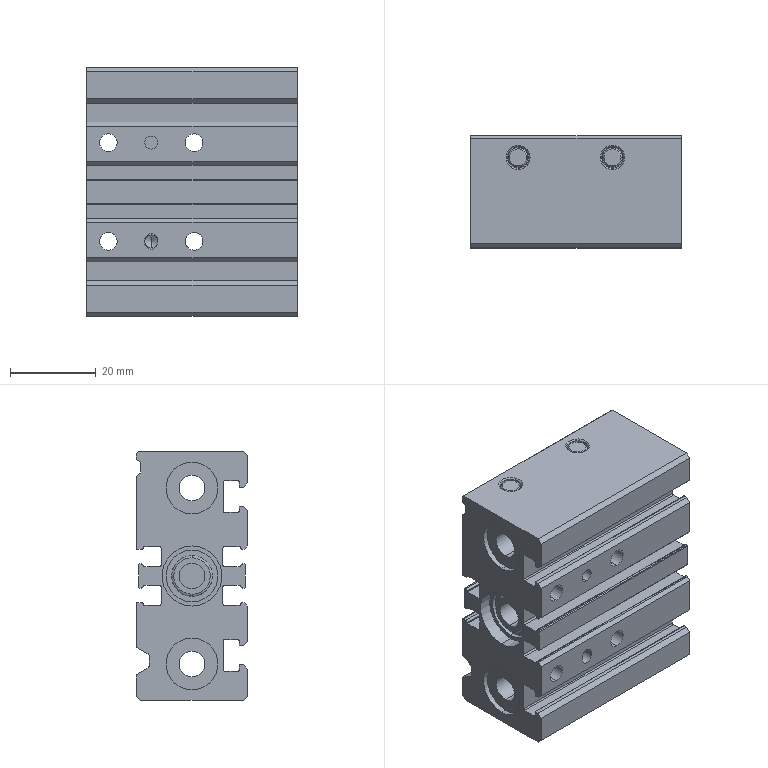Part | SolidWorks | features BaseBody 1 | 1 solid | 281 faces | box 49 x 26 x 58 mm | volume 50658 mm3 | cylinder 126 | plane 101 | cone 52 | spline 2 | commonest cylinder face diameters 0.8 x20 3 x14 0.4 x12 4.134 x12 12 x10 3.242 x8